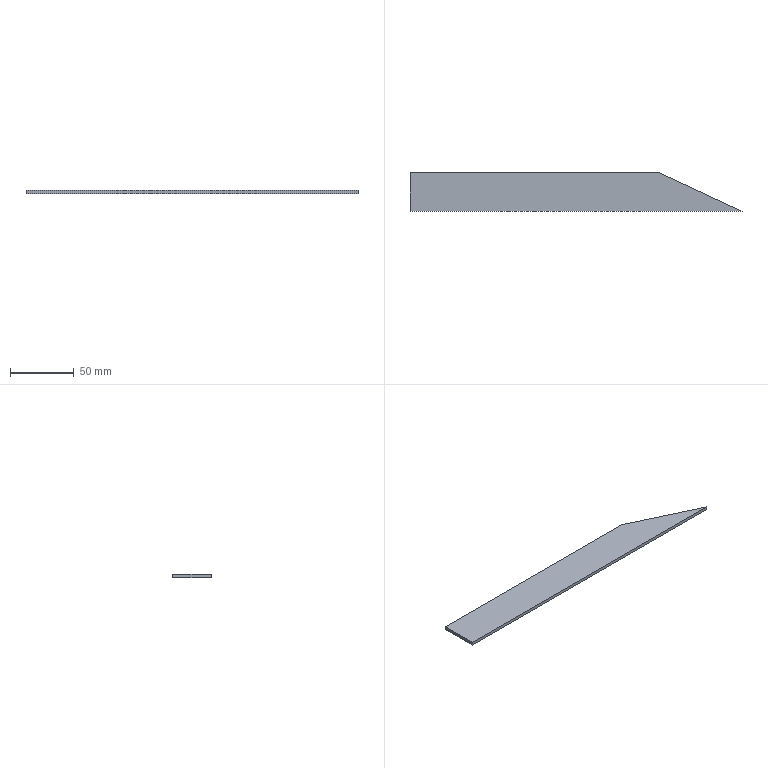Part | SolidWorks | features FlatPattern 1, SMBaseFlange 1, SheetMetal 1 | 1 solid | 6 faces | box 260 x 30 x 2.5 mm | volume 17087 mm3 | plane 6
STEP:
#1=CARTESIAN_POINT('',(0.,0.,0.));
#2=VERTEX_POINT('',#1);
#3=CARTESIAN_POINT('',(260.,0.,0.));
#4=VERTEX_POINT('',#3);
#5=CARTESIAN_POINT('',(260.,0.,0.));
#6=DIRECTION('',(1.,0.,0.));
#7=VECTOR('',#6,1000.);
#8=LINE('',#5,#7);
#9=EDGE_CURVE('',#2,#4,#8,.T.);
#10=ORIENTED_EDGE('',*,*,#9,.F.);
#11=CARTESIAN_POINT('',(0.,0.,-2.5));
#12=VERTEX_POINT('',#11);
#13=CARTESIAN_POINT('',(0.,0.,-2.5));
#14=DIRECTION('',(0.,0.,1.));
#15=VECTOR('',#14,1000.);
#16=LINE('',#13,#15);
#17=EDGE_CURVE('',#12,#2,#16,.T.);
#18=ORIENTED_EDGE('',*,*,#17,.F.);
#19=CARTESIAN_POINT('',(260.,0.,-2.5));
#20=VERTEX_POINT('',#19);
#21=CARTESIAN_POINT('',(260.,0.,-2.5));
#22=DIRECTION('',(1.,0.,0.));
#23=VECTOR('',#22,1000.);
#24=LINE('',#21,#23);
#25=EDGE_CURVE('',#12,#20,#24,.T.);
#26=ORIENTED_EDGE('',*,*,#25,.T.);
#27=CARTESIAN_POINT('',(260.,0.,-2.5));
#28=DIRECTION('',(0.,0.,1.));
#29=VECTOR('',#28,1000.);
#30=LINE('',#27,#29);
#31=EDGE_CURVE('',#20,#4,#30,.T.);
#32=ORIENTED_EDGE('',*,*,#31,.T.);
#33=EDGE_LOOP('',(#10,#18,#26,#32));
#34=FACE_OUTER_BOUND('',#33,.T.);
#35=CARTESIAN_POINT('',(260.,0.,-2.5));
#36=DIRECTION('',(0.,-1.,0.));
#37=DIRECTION('',(1.,0.,0.));
#38=AXIS2_PLACEMENT_3D('',#35,#36,#37);
#39=PLANE('',#38);
#40=ADVANCED_FACE('',(#34),#39,.T.);
#41=CARTESIAN_POINT('',(0.,30.,0.));
#42=VERTEX_POINT('',#41);
#43=CARTESIAN_POINT('',(0.,0.,0.));
#44=DIRECTION('',(0.,-1.,0.));
#45=VECTOR('',#44,1000.);
#46=LINE('',#43,#45);
#47=EDGE_CURVE('',#42,#2,#46,.T.);
#48=ORIENTED_EDGE('',*,*,#47,.F.);
#49=CARTESIAN_POINT('',(0.,30.,-2.5));
#50=VERTEX_POINT('',#49);
#51=CARTESIAN_POINT('',(0.,30.,-2.5));
#52=DIRECTION('',(0.,0.,1.));
#53=VECTOR('',#52,1000.);
#54=LINE('',#51,#53);
#55=EDGE_CURVE('',#50,#42,#54,.T.);
#56=ORIENTED_EDGE('',*,*,#55,.F.);
#57=CARTESIAN_POINT('',(0.,0.,-2.5));
#58=DIRECTION('',(0.,-1.,0.));
#59=VECTOR('',#58,1000.);
#60=LINE('',#57,#59);
#61=EDGE_CURVE('',#50,#12,#60,.T.);
#62=ORIENTED_EDGE('',*,*,#61,.T.);
#63=ORIENTED_EDGE('',*,*,#17,.T.);
#64=EDGE_LOOP('',(#48,#56,#62,#63));
#65=FACE_OUTER_BOUND('',#64,.T.);
#66=CARTESIAN_POINT('',(0.,0.,-2.5));
#67=DIRECTION('',(-1.,0.,0.));
#68=DIRECTION('',(0.,0.,1.));
#69=AXIS2_PLACEMENT_3D('',#66,#67,#68);
#70=PLANE('',#69);
#71=ADVANCED_FACE('',(#65),#70,.T.);
#72=CARTESIAN_POINT('',(195.665,30.,0.));
#73=VERTEX_POINT('',#72);
#74=CARTESIAN_POINT('',(0.,30.,0.));
#75=DIRECTION('',(-1.,0.,0.));
#76=VECTOR('',#75,1000.);
#77=LINE('',#74,#76);
#78=EDGE_CURVE('',#73,#42,#77,.T.);
#79=ORIENTED_EDGE('',*,*,#78,.F.);
#80=CARTESIAN_POINT('',(195.665,30.,-2.5));
#81=VERTEX_POINT('',#80);
#82=CARTESIAN_POINT('',(195.665,30.,-2.5));
#83=DIRECTION('',(0.,0.,1.));
#84=VECTOR('',#83,1000.);
#85=LINE('',#82,#84);
#86=EDGE_CURVE('',#81,#73,#85,.T.);
#87=ORIENTED_EDGE('',*,*,#86,.F.);
#88=CARTESIAN_POINT('',(0.,30.,-2.5));
#89=DIRECTION('',(-1.,0.,0.));
#90=VECTOR('',#89,1000.);
#91=LINE('',#88,#90);
#92=EDGE_CURVE('',#81,#50,#91,.T.);
#93=ORIENTED_EDGE('',*,*,#92,.T.);
#94=ORIENTED_EDGE('',*,*,#55,.T.);
#95=EDGE_LOOP('',(#79,#87,#93,#94));
#96=FACE_OUTER_BOUND('',#95,.T.);
#97=CARTESIAN_POINT('',(0.,30.,-2.5));
#98=DIRECTION('',(0.,1.,0.));
#99=DIRECTION('',(0.,0.,1.));
#100=AXIS2_PLACEMENT_3D('',#97,#98,#99);
#101=PLANE('',#100);
#102=ADVANCED_FACE('',(#96),#101,.T.);
#103=CARTESIAN_POINT('',(195.665,30.,0.));
#104=DIRECTION('',(-0.9063,0.4226,0.));
#105=VECTOR('',#104,1000.);
#106=LINE('',#103,#105);
#107=EDGE_CURVE('',#4,#73,#106,.T.);
#108=ORIENTED_EDGE('',*,*,#107,.F.);
#109=ORIENTED_EDGE('',*,*,#31,.F.);
#110=CARTESIAN_POINT('',(195.665,30.,-2.5));
#111=DIRECTION('',(-0.9063,0.4226,0.));
#112=VECTOR('',#111,1000.);
#113=LINE('',#110,#112);
#114=EDGE_CURVE('',#20,#81,#113,.T.);
#115=ORIENTED_EDGE('',*,*,#114,.T.);
#116=ORIENTED_EDGE('',*,*,#86,.T.);
#117=EDGE_LOOP('',(#108,#109,#115,#116));
#118=FACE_OUTER_BOUND('',#117,.T.);
#119=CARTESIAN_POINT('',(195.665,30.,-2.5));
#120=DIRECTION('',(0.4226,0.9063,0.));
#121=DIRECTION('',(-0.9063,0.4226,0.));
#122=AXIS2_PLACEMENT_3D('',#119,#120,#121);
#123=PLANE('',#122);
#124=ADVANCED_FACE('',(#118),#123,.T.);
#125=ORIENTED_EDGE('',*,*,#25,.F.);
#126=ORIENTED_EDGE('',*,*,#61,.F.);
#127=ORIENTED_EDGE('',*,*,#92,.F.);
#128=ORIENTED_EDGE('',*,*,#114,.F.);
#129=EDGE_LOOP('',(#125,#126,#127,#128));
#130=FACE_OUTER_BOUND('',#129,.T.);
#131=CARTESIAN_POINT('',(0.,0.,-2.5));
#132=DIRECTION('',(0.,0.,-1.));
#133=DIRECTION('',(-1.,0.,0.));
#134=AXIS2_PLACEMENT_3D('',#131,#132,#133);
#135=PLANE('',#134);
#136=ADVANCED_FACE('',(#130),#135,.T.);
#137=ORIENTED_EDGE('',*,*,#9,.T.);
#138=ORIENTED_EDGE('',*,*,#107,.T.);
#139=ORIENTED_EDGE('',*,*,#78,.T.);
#140=ORIENTED_EDGE('',*,*,#47,.T.);
#141=EDGE_LOOP('',(#137,#138,#139,#140));
#142=FACE_OUTER_BOUND('',#141,.T.);
#143=CARTESIAN_POINT('',(0.,0.,0.));
#144=DIRECTION('',(0.,0.,-1.));
#145=DIRECTION('',(-1.,0.,0.));
#146=AXIS2_PLACEMENT_3D('',#143,#144,#145);
#147=PLANE('',#146);
#148=ADVANCED_FACE('',(#142),#147,.F.);
#149=CLOSED_SHELL('',(#40,#71,#102,#124,#136,#148));
#150=MANIFOLD_SOLID_BREP('',#149);
#151=CARTESIAN_POINT('',(0.,0.,0.));
#152=DIRECTION('',(0.,0.,1.));
#153=DIRECTION('',(1.,0.,0.));
#154=AXIS2_PLACEMENT_3D('',#151,#152,#153);
#155=(LENGTH_UNIT()NAMED_UNIT(*)SI_UNIT(.MILLI.,.METRE.));
#156=UNCERTAINTY_MEASURE_WITH_UNIT(LENGTH_MEASURE(0.00001),#155,'','');
#157=(NAMED_UNIT(*)PLANE_ANGLE_UNIT()SI_UNIT($,.RADIAN.));
#158=(NAMED_UNIT(*)SI_UNIT($,.STERADIAN.)SOLID_ANGLE_UNIT());
#159=(GEOMETRIC_REPRESENTATION_CONTEXT(3)GLOBAL_UNCERTAINTY_ASSIGNED_CONTEXT((#156))GLOBAL_UNIT_ASSIGNED_CONTEXT((#155,#157,#158))REPRESENTATION_CONTEXT('',''));
#160=ADVANCED_BREP_SHAPE_REPRESENTATION('',(#150,#154),#159);